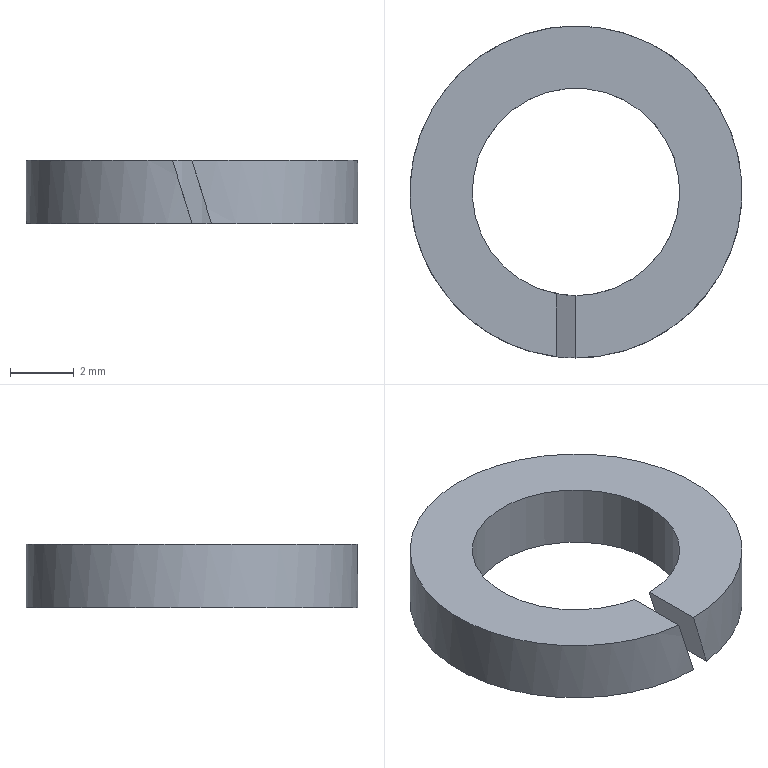Part | STEP file | 1_26 | 1 solid | 6 faces | box 10.4 x 10.4 x 2 mm | volume 101.14 mm3 | plane 4 | cylinder 2 | commonest cylinder face diameters 6.5 x1 10.4 x1
STEP:
#1=CARTESIAN_POINT('',(0.,0.,0.));
#2=DIRECTION('',(0.,0.,1.));
#3=DIRECTION('',(1.,0.,0.));
#4=AXIS2_PLACEMENT_3D('',#1,#2,#3);
#5=CARTESIAN_POINT('',(0.6118,-3.192,0.));
#6=VERTEX_POINT('',#5);
#7=CARTESIAN_POINT('',(0.,-3.25,2.));
#8=VERTEX_POINT('',#7);
#9=CARTESIAN_POINT('',(0.,0.,2.));
#10=DIRECTION('',(-0.9563,0.,-0.2925));
#11=DIRECTION('',(0.2925,0.,-0.9563));
#12=AXIS2_PLACEMENT_3D('',#9,#10,#11);
#13=ELLIPSE('',#12,11.111,3.25);
#14=CARTESIAN_POINT('',(0.,0.,1.));
#15=DIRECTION('',(0.,0.,-1.));
#16=DIRECTION('',(1.,0.,0.));
#17=AXIS2_PLACEMENT_3D('',#14,#15,#16);
#18=CYLINDRICAL_SURFACE('',#17,3.25);
#19=CARTESIAN_POINT('',(7.665,1.));
#20=CARTESIAN_POINT('',(7.854,-1.));
#21=B_SPLINE_CURVE_WITH_KNOTS('',1,(#19,#20),.UNSPECIFIED.,.F.,.F.,(2,2),(1.381,1.571),.PIECEWISE_BEZIER_KNOTS.);
#22=(GEOMETRIC_REPRESENTATION_CONTEXT(2)PARAMETRIC_REPRESENTATION_CONTEXT()REPRESENTATION_CONTEXT('',''));
#23=DEFINITIONAL_REPRESENTATION('',(#21),#22);
#24=PCURVE('',#18,#23);
#25=CARTESIAN_POINT('',(0.,-3.055,2.));
#26=DIRECTION('',(0.9563,0.,0.2925));
#27=DIRECTION('',(0.2925,0.,-0.9563));
#28=AXIS2_PLACEMENT_3D('',#25,#26,#27);
#29=PLANE('',#28);
#30=CARTESIAN_POINT('',(11.111,3.055));
#31=CARTESIAN_POINT('',(11.111,-2.574));
#32=CARTESIAN_POINT('',(-5.555,0.2404));
#33=CARTESIAN_POINT('',(-22.222,3.055));
#34=CARTESIAN_POINT('',(-5.555,5.87));
#35=CARTESIAN_POINT('',(11.111,8.684));
#36=CARTESIAN_POINT('',(11.111,3.055));
#37=(BOUNDED_CURVE()B_SPLINE_CURVE(2,(#30,#31,#32,#33,#34,#35,#36),.UNSPECIFIED.,.T.,.F.)B_SPLINE_CURVE_WITH_KNOTS((1,2,2,2,2,1),(-2.094,0.,2.094,4.189,6.283,8.378),.UNSPECIFIED.)CURVE()GEOMETRIC_REPRESENTATION_ITEM()RATIONAL_B_SPLINE_CURVE((1.,0.5,1.,0.5,1.,0.5,1.))REPRESENTATION_ITEM(''));
#38=(GEOMETRIC_REPRESENTATION_CONTEXT(2)PARAMETRIC_REPRESENTATION_CONTEXT()REPRESENTATION_CONTEXT('',''));
#39=DEFINITIONAL_REPRESENTATION('',(#37),#38);
#40=PCURVE('',#29,#39);
#41=SURFACE_CURVE('',#13,(#24,#40),.PCURVE_S1.);
#42=EDGE_CURVE('',#6,#8,#41,.T.);
#43=ORIENTED_EDGE('',*,*,#42,.F.);
#44=CARTESIAN_POINT('',(0.,-3.25,0.));
#45=VERTEX_POINT('',#44);
#46=CARTESIAN_POINT('',(0.,0.,0.));
#47=DIRECTION('',(0.,0.,1.));
#48=DIRECTION('',(1.,0.,0.));
#49=AXIS2_PLACEMENT_3D('',#46,#47,#48);
#50=CIRCLE('',#49,3.25);
#51=CARTESIAN_POINT('',(12.566,1.));
#52=DIRECTION('',(-1.,0.));
#53=VECTOR('',#52,1.);
#54=LINE('',#51,#53);
#55=(GEOMETRIC_REPRESENTATION_CONTEXT(2)PARAMETRIC_REPRESENTATION_CONTEXT()REPRESENTATION_CONTEXT('',''));
#56=DEFINITIONAL_REPRESENTATION('',(#54),#55);
#57=PCURVE('',#18,#56);
#58=CARTESIAN_POINT('',(4.225,0.,0.));
#59=DIRECTION('',(0.,0.,-1.));
#60=DIRECTION('',(-1.,0.,0.));
#61=AXIS2_PLACEMENT_3D('',#58,#59,#60);
#62=PLANE('',#61);
#63=CARTESIAN_POINT('',(0.975,0.));
#64=CARTESIAN_POINT('',(0.975,5.629));
#65=CARTESIAN_POINT('',(5.85,2.815));
#66=CARTESIAN_POINT('',(10.725,0.));
#67=CARTESIAN_POINT('',(5.85,-2.815));
#68=CARTESIAN_POINT('',(0.975,-5.629));
#69=CARTESIAN_POINT('',(0.975,0.));
#70=(BOUNDED_CURVE()B_SPLINE_CURVE(2,(#63,#64,#65,#66,#67,#68,#69),.UNSPECIFIED.,.T.,.F.)B_SPLINE_CURVE_WITH_KNOTS((1,2,2,2,2,1),(-2.094,0.,2.094,4.189,6.283,8.378),.UNSPECIFIED.)CURVE()GEOMETRIC_REPRESENTATION_ITEM()RATIONAL_B_SPLINE_CURVE((1.,0.5,1.,0.5,1.,0.5,1.))REPRESENTATION_ITEM(''));
#71=(GEOMETRIC_REPRESENTATION_CONTEXT(2)PARAMETRIC_REPRESENTATION_CONTEXT()REPRESENTATION_CONTEXT('',''));
#72=DEFINITIONAL_REPRESENTATION('',(#70),#71);
#73=PCURVE('',#62,#72);
#74=SURFACE_CURVE('',#50,(#57,#73),.PCURVE_S1.);
#75=EDGE_CURVE('',#6,#45,#74,.T.);
#76=ORIENTED_EDGE('',*,*,#75,.T.);
#77=CARTESIAN_POINT('',(-0.6118,-3.192,2.));
#78=VERTEX_POINT('',#77);
#79=CARTESIAN_POINT('',(0.,0.,0.));
#80=DIRECTION('',(0.9563,0.,0.2925));
#81=DIRECTION('',(0.2925,0.,-0.9563));
#82=AXIS2_PLACEMENT_3D('',#79,#80,#81);
#83=ELLIPSE('',#82,11.111,3.25);
#84=CARTESIAN_POINT('',(1.76,-1.));
#85=CARTESIAN_POINT('',(1.571,1.));
#86=B_SPLINE_CURVE_WITH_KNOTS('',1,(#84,#85),.UNSPECIFIED.,.F.,.F.,(2,2),(4.523,4.712),.PIECEWISE_BEZIER_KNOTS.);
#87=(GEOMETRIC_REPRESENTATION_CONTEXT(2)PARAMETRIC_REPRESENTATION_CONTEXT()REPRESENTATION_CONTEXT('',''));
#88=DEFINITIONAL_REPRESENTATION('',(#86),#87);
#89=PCURVE('',#18,#88);
#90=CARTESIAN_POINT('',(0.,-3.055,0.));
#91=DIRECTION('',(-0.9563,0.,-0.2925));
#92=DIRECTION('',(-0.2925,0.,0.9563));
#93=AXIS2_PLACEMENT_3D('',#90,#91,#92);
#94=PLANE('',#93);
#95=CARTESIAN_POINT('',(-11.111,3.055));
#96=CARTESIAN_POINT('',(-11.111,8.684));
#97=CARTESIAN_POINT('',(5.555,5.87));
#98=CARTESIAN_POINT('',(22.222,3.055));
#99=CARTESIAN_POINT('',(5.555,0.2404));
#100=CARTESIAN_POINT('',(-11.111,-2.574));
#101=CARTESIAN_POINT('',(-11.111,3.055));
#102=(BOUNDED_CURVE()B_SPLINE_CURVE(2,(#95,#96,#97,#98,#99,#100,#101),.UNSPECIFIED.,.T.,.F.)B_SPLINE_CURVE_WITH_KNOTS((1,2,2,2,2,1),(-2.094,0.,2.094,4.189,6.283,8.378),.UNSPECIFIED.)CURVE()GEOMETRIC_REPRESENTATION_ITEM()RATIONAL_B_SPLINE_CURVE((1.,0.5,1.,0.5,1.,0.5,1.))REPRESENTATION_ITEM(''));
#103=(GEOMETRIC_REPRESENTATION_CONTEXT(2)PARAMETRIC_REPRESENTATION_CONTEXT()REPRESENTATION_CONTEXT('',''));
#104=DEFINITIONAL_REPRESENTATION('',(#102),#103);
#105=PCURVE('',#94,#104);
#106=SURFACE_CURVE('',#83,(#89,#105),.PCURVE_S1.);
#107=EDGE_CURVE('',#78,#45,#106,.T.);
#108=ORIENTED_EDGE('',*,*,#107,.F.);
#109=CARTESIAN_POINT('',(0.,0.,2.));
#110=DIRECTION('',(0.,0.,-1.));
#111=DIRECTION('',(1.,0.,0.));
#112=AXIS2_PLACEMENT_3D('',#109,#110,#111);
#113=CIRCLE('',#112,3.25);
#114=CARTESIAN_POINT('',(0.,-1.));
#115=DIRECTION('',(1.,0.));
#116=VECTOR('',#115,1.);
#117=LINE('',#114,#116);
#118=(GEOMETRIC_REPRESENTATION_CONTEXT(2)PARAMETRIC_REPRESENTATION_CONTEXT()REPRESENTATION_CONTEXT('',''));
#119=DEFINITIONAL_REPRESENTATION('',(#117),#118);
#120=PCURVE('',#18,#119);
#121=CARTESIAN_POINT('',(4.225,0.,2.));
#122=DIRECTION('',(0.,0.,1.));
#123=DIRECTION('',(1.,0.,0.));
#124=AXIS2_PLACEMENT_3D('',#121,#122,#123);
#125=PLANE('',#124);
#126=CARTESIAN_POINT('',(-0.975,0.));
#127=CARTESIAN_POINT('',(-0.975,-5.629));
#128=CARTESIAN_POINT('',(-5.85,-2.815));
#129=CARTESIAN_POINT('',(-10.725,0.));
#130=CARTESIAN_POINT('',(-5.85,2.815));
#131=CARTESIAN_POINT('',(-0.975,5.629));
#132=CARTESIAN_POINT('',(-0.975,0.));
#133=(BOUNDED_CURVE()B_SPLINE_CURVE(2,(#126,#127,#128,#129,#130,#131,#132),.UNSPECIFIED.,.T.,.F.)B_SPLINE_CURVE_WITH_KNOTS((1,2,2,2,2,1),(-2.094,0.,2.094,4.189,6.283,8.378),.UNSPECIFIED.)CURVE()GEOMETRIC_REPRESENTATION_ITEM()RATIONAL_B_SPLINE_CURVE((1.,0.5,1.,0.5,1.,0.5,1.))REPRESENTATION_ITEM(''));
#134=(GEOMETRIC_REPRESENTATION_CONTEXT(2)PARAMETRIC_REPRESENTATION_CONTEXT()REPRESENTATION_CONTEXT('',''));
#135=DEFINITIONAL_REPRESENTATION('',(#133),#134);
#136=PCURVE('',#125,#135);
#137=SURFACE_CURVE('',#113,(#120,#136),.PCURVE_S1.);
#138=EDGE_CURVE('',#78,#8,#137,.T.);
#139=ORIENTED_EDGE('',*,*,#138,.T.);
#140=EDGE_LOOP('',(#43,#76,#108,#139));
#141=FACE_BOUND('',#140,.F.);
#142=ADVANCED_FACE('',(#141),#18,.F.);
#143=CARTESIAN_POINT('',(0.,-5.2,2.));
#144=VERTEX_POINT('',#143);
#145=CARTESIAN_POINT('',(0.,-3.25,2.));
#146=DIRECTION('',(0.,-1.,0.));
#147=VECTOR('',#146,1.);
#148=LINE('',#145,#147);
#149=CARTESIAN_POINT('',(-4.225,-3.25));
#150=DIRECTION('',(0.,-1.));
#151=VECTOR('',#150,1.);
#152=LINE('',#149,#151);
#153=(GEOMETRIC_REPRESENTATION_CONTEXT(2)PARAMETRIC_REPRESENTATION_CONTEXT()REPRESENTATION_CONTEXT('',''));
#154=DEFINITIONAL_REPRESENTATION('',(#152),#153);
#155=PCURVE('',#125,#154);
#156=CARTESIAN_POINT('',(0.,-0.195));
#157=DIRECTION('',(0.,-1.));
#158=VECTOR('',#157,1.);
#159=LINE('',#156,#158);
#160=(GEOMETRIC_REPRESENTATION_CONTEXT(2)PARAMETRIC_REPRESENTATION_CONTEXT()REPRESENTATION_CONTEXT('',''));
#161=DEFINITIONAL_REPRESENTATION('',(#159),#160);
#162=PCURVE('',#29,#161);
#163=SURFACE_CURVE('',#148,(#155,#162),.PCURVE_S1.);
#164=EDGE_CURVE('',#8,#144,#163,.T.);
#165=ORIENTED_EDGE('',*,*,#164,.T.);
#166=CARTESIAN_POINT('',(-0.6118,-5.164,2.));
#167=VERTEX_POINT('',#166);
#168=CARTESIAN_POINT('',(0.000000002,-0.000000002,2.));
#169=DIRECTION('',(0.,0.,1.));
#170=DIRECTION('',(1.,0.,0.));
#171=AXIS2_PLACEMENT_3D('',#168,#169,#170);
#172=CIRCLE('',#171,5.2);
#173=CARTESIAN_POINT('',(-4.225,-0.000000002));
#174=DIRECTION('',(1.,0.));
#175=AXIS2_PLACEMENT_2D('',#173,#174);
#176=CIRCLE('',#175,5.2);
#177=(GEOMETRIC_REPRESENTATION_CONTEXT(2)PARAMETRIC_REPRESENTATION_CONTEXT()REPRESENTATION_CONTEXT('',''));
#178=DEFINITIONAL_REPRESENTATION('',(#176),#177);
#179=PCURVE('',#125,#178);
#180=CARTESIAN_POINT('',(0.,0.,1.));
#181=DIRECTION('',(0.,0.,-1.));
#182=DIRECTION('',(1.,0.,0.));
#183=AXIS2_PLACEMENT_3D('',#180,#181,#182);
#184=CYLINDRICAL_SURFACE('',#183,5.2);
#185=CARTESIAN_POINT('',(12.566,-1.));
#186=DIRECTION('',(-1.,0.));
#187=VECTOR('',#186,1.);
#188=LINE('',#185,#187);
#189=(GEOMETRIC_REPRESENTATION_CONTEXT(2)PARAMETRIC_REPRESENTATION_CONTEXT()REPRESENTATION_CONTEXT('',''));
#190=DEFINITIONAL_REPRESENTATION('',(#188),#189);
#191=PCURVE('',#184,#190);
#192=SURFACE_CURVE('',#172,(#179,#191),.PCURVE_S1.);
#193=EDGE_CURVE('',#144,#167,#192,.T.);
#194=ORIENTED_EDGE('',*,*,#193,.T.);
#195=CARTESIAN_POINT('',(-0.6118,-5.164,2.));
#196=DIRECTION('',(0.,1.,0.));
#197=VECTOR('',#196,1.);
#198=LINE('',#195,#197);
#199=CARTESIAN_POINT('',(-4.837,-5.164));
#200=DIRECTION('',(0.,1.));
#201=VECTOR('',#200,1.);
#202=LINE('',#199,#201);
#203=(GEOMETRIC_REPRESENTATION_CONTEXT(2)PARAMETRIC_REPRESENTATION_CONTEXT()REPRESENTATION_CONTEXT('',''));
#204=DEFINITIONAL_REPRESENTATION('',(#202),#203);
#205=PCURVE('',#125,#204);
#206=CARTESIAN_POINT('',(2.091,-2.109));
#207=DIRECTION('',(0.,1.));
#208=VECTOR('',#207,1.);
#209=LINE('',#206,#208);
#210=(GEOMETRIC_REPRESENTATION_CONTEXT(2)PARAMETRIC_REPRESENTATION_CONTEXT()REPRESENTATION_CONTEXT('',''));
#211=DEFINITIONAL_REPRESENTATION('',(#209),#210);
#212=PCURVE('',#94,#211);
#213=SURFACE_CURVE('',#198,(#205,#212),.PCURVE_S1.);
#214=EDGE_CURVE('',#167,#78,#213,.T.);
#215=ORIENTED_EDGE('',*,*,#214,.T.);
#216=ORIENTED_EDGE('',*,*,#138,.T.);
#217=EDGE_LOOP('',(#165,#194,#215,#216));
#218=FACE_BOUND('',#217,.T.);
#219=ADVANCED_FACE('',(#218),#125,.T.);
#220=ORIENTED_EDGE('',*,*,#107,.F.);
#221=ORIENTED_EDGE('',*,*,#214,.F.);
#222=CARTESIAN_POINT('',(0.,-5.2,0.));
#223=VERTEX_POINT('',#222);
#224=CARTESIAN_POINT('',(-0.01082,-0.1835,0.03538));
#225=DIRECTION('',(-0.9563,0.,-0.2925));
#226=DIRECTION('',(0.2925,-0.0006634,-0.9563));
#227=AXIS2_PLACEMENT_3D('',#224,#225,#226);
#228=ELLIPSE('',#227,17.46,5.017);
#229=CARTESIAN_POINT('',(0.037,2.872));
#230=DIRECTION('',(-1.,-0.0006634));
#231=AXIS2_PLACEMENT_2D('',#229,#230);
#232=ELLIPSE('',#231,17.46,5.017);
#233=(GEOMETRIC_REPRESENTATION_CONTEXT(2)PARAMETRIC_REPRESENTATION_CONTEXT()REPRESENTATION_CONTEXT('',''));
#234=DEFINITIONAL_REPRESENTATION('',(#232),#233);
#235=PCURVE('',#94,#234);
#236=CARTESIAN_POINT('',(1.571,1.));
#237=CARTESIAN_POINT('',(1.689,-1.));
#238=B_SPLINE_CURVE_WITH_KNOTS('',1,(#236,#237),.UNSPECIFIED.,.F.,.F.,(2,2),(1.568,1.689),.PIECEWISE_BEZIER_KNOTS.);
#239=(GEOMETRIC_REPRESENTATION_CONTEXT(2)PARAMETRIC_REPRESENTATION_CONTEXT()REPRESENTATION_CONTEXT('',''));
#240=DEFINITIONAL_REPRESENTATION('',(#238),#239);
#241=PCURVE('',#184,#240);
#242=SURFACE_CURVE('',#228,(#235,#241),.PCURVE_S1.);
#243=EDGE_CURVE('',#223,#167,#242,.T.);
#244=ORIENTED_EDGE('',*,*,#243,.F.);
#245=CARTESIAN_POINT('',(0.,-3.25,0.));
#246=DIRECTION('',(0.,-1.,0.));
#247=VECTOR('',#246,1.);
#248=LINE('',#245,#247);
#249=CARTESIAN_POINT('',(0.,-0.195));
#250=DIRECTION('',(0.,-1.));
#251=VECTOR('',#250,1.);
#252=LINE('',#249,#251);
#253=(GEOMETRIC_REPRESENTATION_CONTEXT(2)PARAMETRIC_REPRESENTATION_CONTEXT()REPRESENTATION_CONTEXT('',''));
#254=DEFINITIONAL_REPRESENTATION('',(#252),#253);
#255=PCURVE('',#94,#254);
#256=CARTESIAN_POINT('',(4.225,-3.25));
#257=DIRECTION('',(0.,-1.));
#258=VECTOR('',#257,1.);
#259=LINE('',#256,#258);
#260=(GEOMETRIC_REPRESENTATION_CONTEXT(2)PARAMETRIC_REPRESENTATION_CONTEXT()REPRESENTATION_CONTEXT('',''));
#261=DEFINITIONAL_REPRESENTATION('',(#259),#260);
#262=PCURVE('',#62,#261);
#263=SURFACE_CURVE('',#248,(#255,#262),.PCURVE_S1.);
#264=EDGE_CURVE('',#45,#223,#263,.T.);
#265=ORIENTED_EDGE('',*,*,#264,.F.);
#266=EDGE_LOOP('',(#220,#221,#244,#265));
#267=FACE_BOUND('',#266,.T.);
#268=ADVANCED_FACE('',(#267),#94,.F.);
#269=CARTESIAN_POINT('',(0.6118,-5.164,0.));
#270=VERTEX_POINT('',#269);
#271=CARTESIAN_POINT('',(0.6118,-5.164,0.));
#272=DIRECTION('',(0.,1.,0.));
#273=VECTOR('',#272,1.);
#274=LINE('',#271,#273);
#275=CARTESIAN_POINT('',(3.613,-5.164));
#276=DIRECTION('',(0.,1.));
#277=VECTOR('',#276,1.);
#278=LINE('',#275,#277);
#279=(GEOMETRIC_REPRESENTATION_CONTEXT(2)PARAMETRIC_REPRESENTATION_CONTEXT()REPRESENTATION_CONTEXT('',''));
#280=DEFINITIONAL_REPRESENTATION('',(#278),#279);
#281=PCURVE('',#62,#280);
#282=CARTESIAN_POINT('',(2.091,-2.109));
#283=DIRECTION('',(0.,1.));
#284=VECTOR('',#283,1.);
#285=LINE('',#282,#284);
#286=(GEOMETRIC_REPRESENTATION_CONTEXT(2)PARAMETRIC_REPRESENTATION_CONTEXT()REPRESENTATION_CONTEXT('',''));
#287=DEFINITIONAL_REPRESENTATION('',(#285),#286);
#288=PCURVE('',#29,#287);
#289=SURFACE_CURVE('',#274,(#281,#288),.PCURVE_S1.);
#290=EDGE_CURVE('',#270,#6,#289,.T.);
#291=ORIENTED_EDGE('',*,*,#290,.T.);
#292=ORIENTED_EDGE('',*,*,#75,.T.);
#293=ORIENTED_EDGE('',*,*,#264,.T.);
#294=CARTESIAN_POINT('',(0.,0.,0.));
#295=DIRECTION('',(0.,0.,1.));
#296=DIRECTION('',(0.,-1.,0.));
#297=AXIS2_PLACEMENT_3D('',#294,#295,#296);
#298=CIRCLE('',#297,5.2);
#299=CARTESIAN_POINT('',(4.225,-5.2));
#300=CARTESIAN_POINT('',(-4.782,-5.2));
#301=CARTESIAN_POINT('',(-0.2783,2.6));
#302=CARTESIAN_POINT('',(4.225,10.4));
#303=CARTESIAN_POINT('',(8.728,2.6));
#304=CARTESIAN_POINT('',(13.232,-5.2));
#305=CARTESIAN_POINT('',(4.225,-5.2));
#306=(BOUNDED_CURVE()B_SPLINE_CURVE(2,(#299,#300,#301,#302,#303,#304,#305),.UNSPECIFIED.,.T.,.F.)B_SPLINE_CURVE_WITH_KNOTS((1,2,2,2,2,1),(-2.094,0.,2.094,4.189,6.283,8.378),.UNSPECIFIED.)CURVE()GEOMETRIC_REPRESENTATION_ITEM()RATIONAL_B_SPLINE_CURVE((1.,0.5,1.,0.5,1.,0.5,1.))REPRESENTATION_ITEM(''));
#307=(GEOMETRIC_REPRESENTATION_CONTEXT(2)PARAMETRIC_REPRESENTATION_CONTEXT()REPRESENTATION_CONTEXT('',''));
#308=DEFINITIONAL_REPRESENTATION('',(#306),#307);
#309=PCURVE('',#62,#308);
#310=CARTESIAN_POINT('',(7.854,1.));
#311=DIRECTION('',(-1.,0.));
#312=VECTOR('',#311,1.);
#313=LINE('',#310,#312);
#314=(GEOMETRIC_REPRESENTATION_CONTEXT(2)PARAMETRIC_REPRESENTATION_CONTEXT()REPRESENTATION_CONTEXT('',''));
#315=DEFINITIONAL_REPRESENTATION('',(#313),#314);
#316=PCURVE('',#184,#315);
#317=SURFACE_CURVE('',#298,(#309,#316),.PCURVE_S1.);
#318=EDGE_CURVE('',#270,#223,#317,.T.);
#319=ORIENTED_EDGE('',*,*,#318,.F.);
#320=EDGE_LOOP('',(#291,#292,#293,#319));
#321=FACE_BOUND('',#320,.T.);
#322=ADVANCED_FACE('',(#321),#62,.T.);
#323=ORIENTED_EDGE('',*,*,#42,.F.);
#324=ORIENTED_EDGE('',*,*,#290,.F.);
#325=CARTESIAN_POINT('',(0.01082,-0.1835,1.965));
#326=DIRECTION('',(0.9563,0.,0.2925));
#327=DIRECTION('',(0.2925,0.0006634,-0.9563));
#328=AXIS2_PLACEMENT_3D('',#325,#326,#327);
#329=ELLIPSE('',#328,17.46,5.017);
#330=CARTESIAN_POINT('',(0.037,2.872));
#331=DIRECTION('',(1.,0.0006634));
#332=AXIS2_PLACEMENT_2D('',#330,#331);
#333=ELLIPSE('',#332,17.46,5.017);
#334=(GEOMETRIC_REPRESENTATION_CONTEXT(2)PARAMETRIC_REPRESENTATION_CONTEXT()REPRESENTATION_CONTEXT('',''));
#335=DEFINITIONAL_REPRESENTATION('',(#333),#334);
#336=PCURVE('',#29,#335);
#337=CARTESIAN_POINT('',(7.854,-1.));
#338=CARTESIAN_POINT('',(7.736,1.));
#339=B_SPLINE_CURVE_WITH_KNOTS('',1,(#337,#338),.UNSPECIFIED.,.F.,.F.,(2,2),(4.71,4.83),.PIECEWISE_BEZIER_KNOTS.);
#340=(GEOMETRIC_REPRESENTATION_CONTEXT(2)PARAMETRIC_REPRESENTATION_CONTEXT()REPRESENTATION_CONTEXT('',''));
#341=DEFINITIONAL_REPRESENTATION('',(#339),#340);
#342=PCURVE('',#184,#341);
#343=SURFACE_CURVE('',#329,(#336,#342),.PCURVE_S1.);
#344=EDGE_CURVE('',#144,#270,#343,.T.);
#345=ORIENTED_EDGE('',*,*,#344,.F.);
#346=ORIENTED_EDGE('',*,*,#164,.F.);
#347=EDGE_LOOP('',(#323,#324,#345,#346));
#348=FACE_BOUND('',#347,.T.);
#349=ADVANCED_FACE('',(#348),#29,.F.);
#350=ORIENTED_EDGE('',*,*,#193,.F.);
#351=ORIENTED_EDGE('',*,*,#344,.T.);
#352=ORIENTED_EDGE('',*,*,#318,.T.);
#353=ORIENTED_EDGE('',*,*,#243,.T.);
#354=EDGE_LOOP('',(#350,#351,#352,#353));
#355=FACE_BOUND('',#354,.T.);
#356=ADVANCED_FACE('',(#355),#184,.T.);
#357=CLOSED_SHELL('',(#142,#219,#268,#322,#349,#356));
#358=MANIFOLD_SOLID_BREP('',#357);
#359=(LENGTH_UNIT()NAMED_UNIT(*)SI_UNIT(.MILLI.,.METRE.));
#360=UNCERTAINTY_MEASURE_WITH_UNIT(LENGTH_MEASURE(0.002),#359,'','');
#361=(NAMED_UNIT(*)PLANE_ANGLE_UNIT()SI_UNIT($,.RADIAN.));
#362=(NAMED_UNIT(*)SI_UNIT($,.STERADIAN.)SOLID_ANGLE_UNIT());
#363=(GEOMETRIC_REPRESENTATION_CONTEXT(3)GLOBAL_UNCERTAINTY_ASSIGNED_CONTEXT((#360))GLOBAL_UNIT_ASSIGNED_CONTEXT((#359,#361,#362))REPRESENTATION_CONTEXT('',''));
#364=ADVANCED_BREP_SHAPE_REPRESENTATION('',(#4,#358),#363);